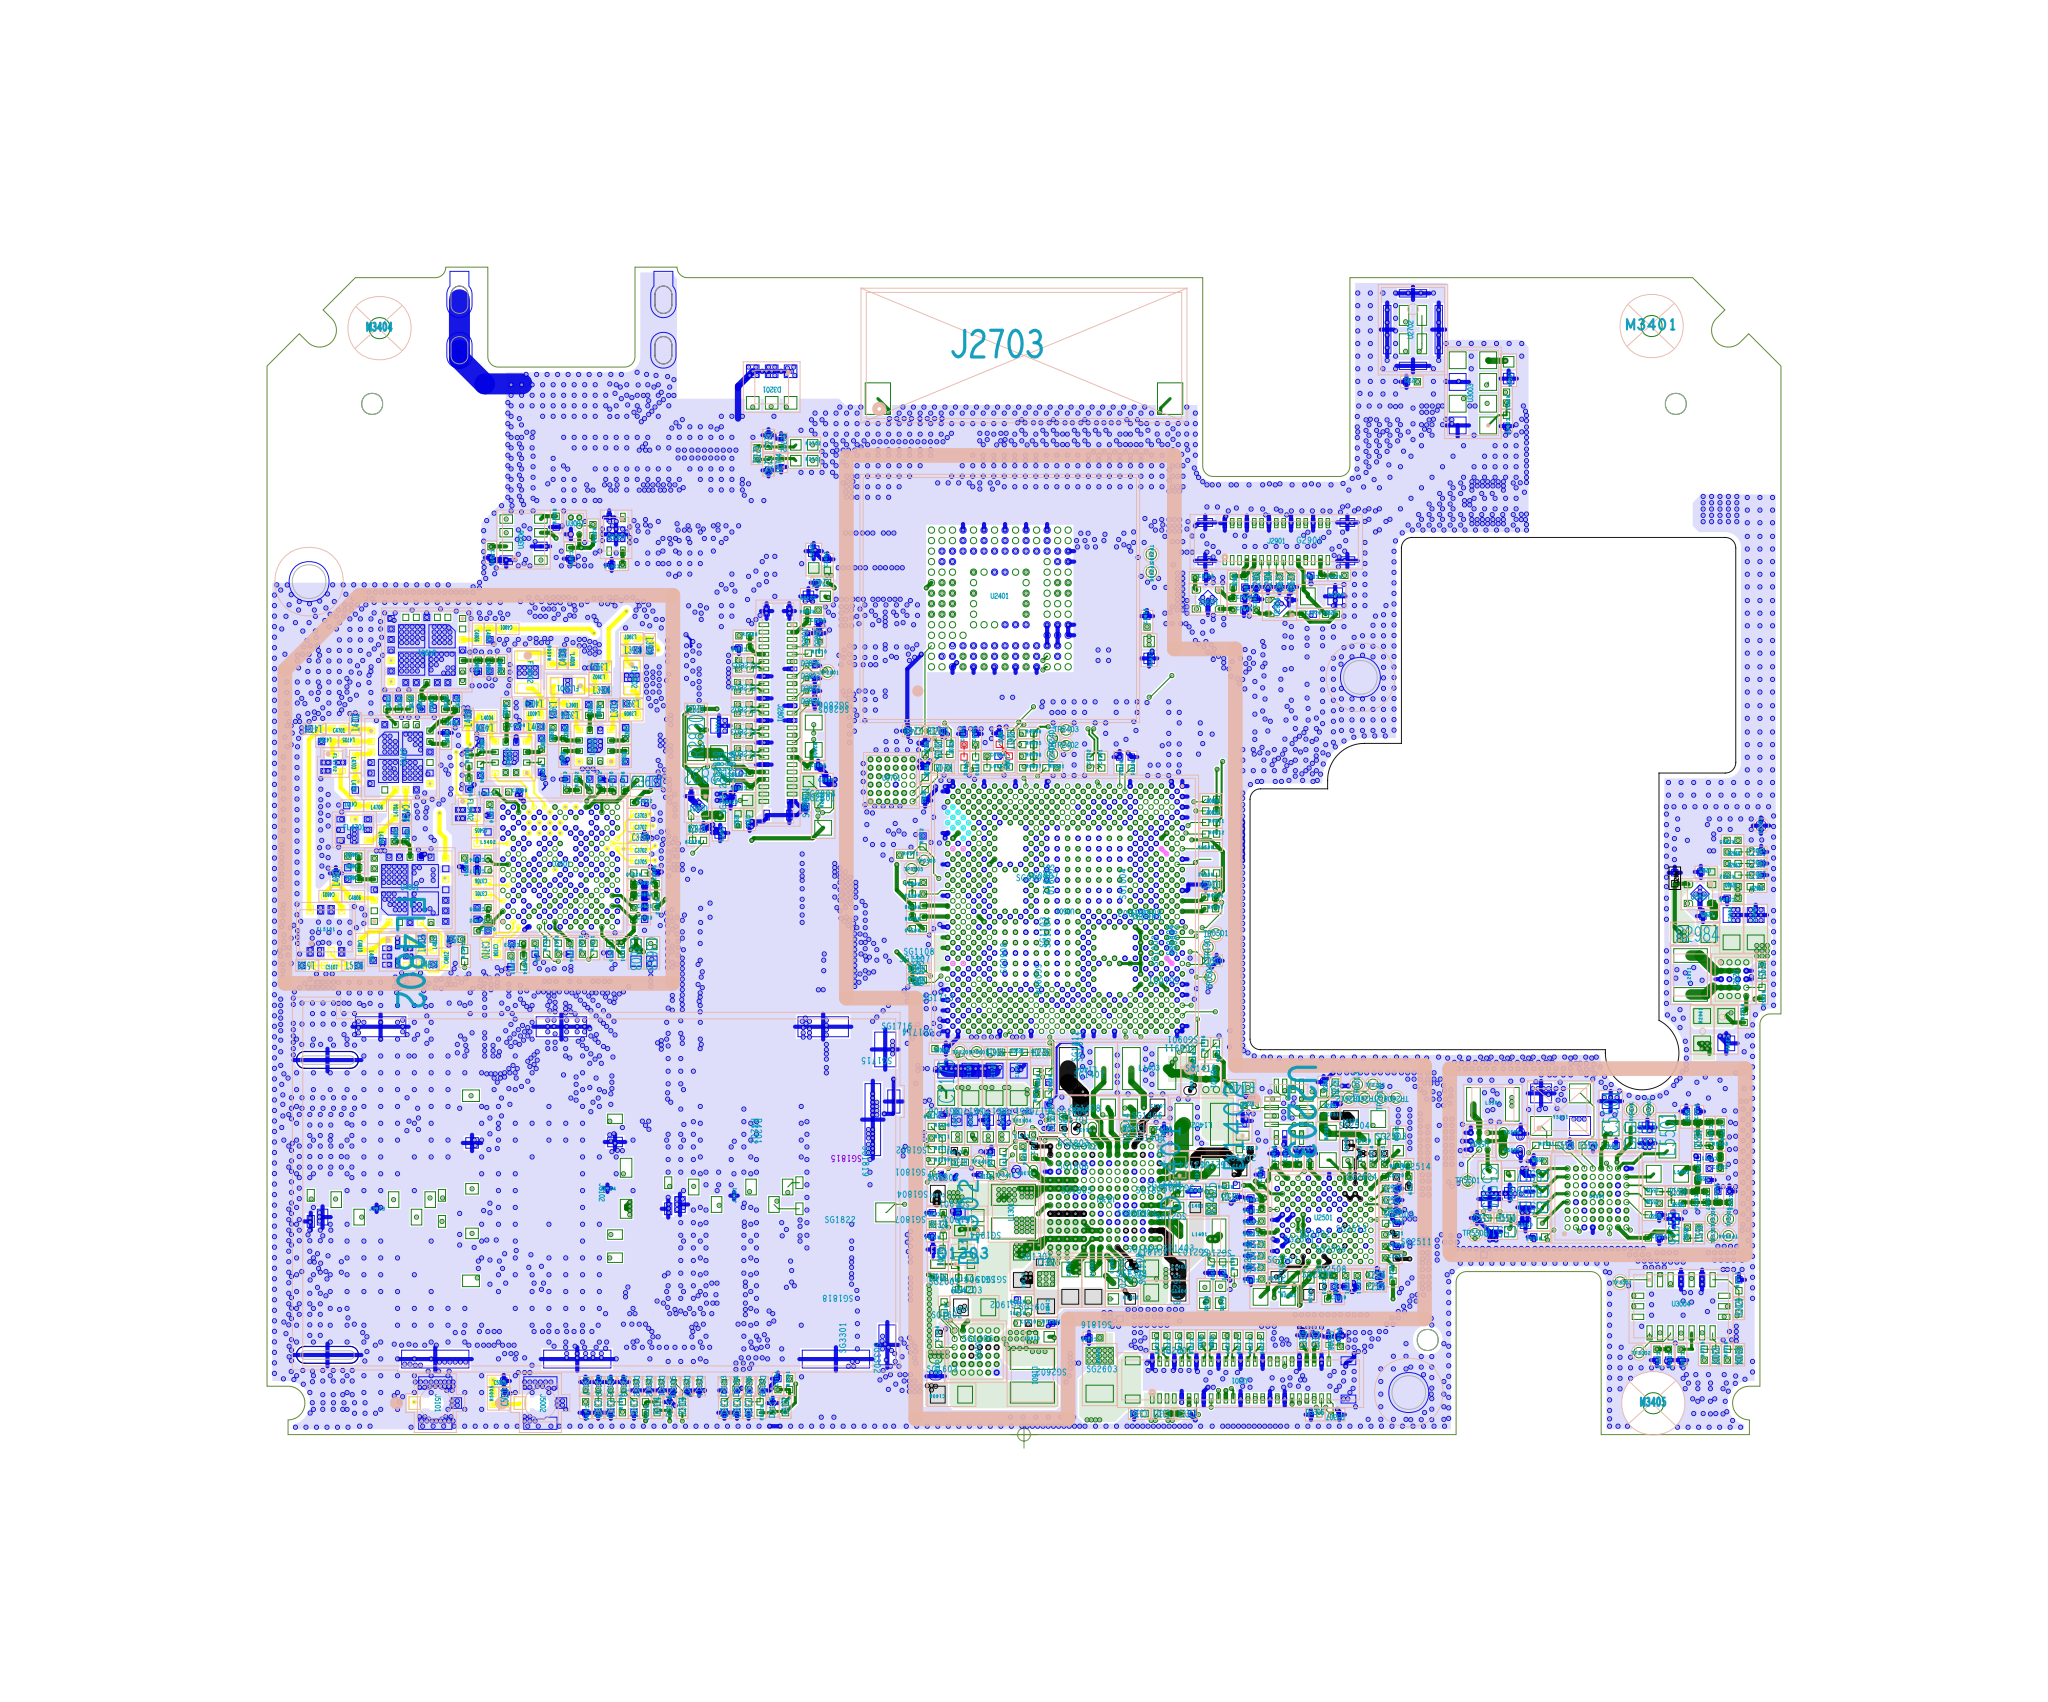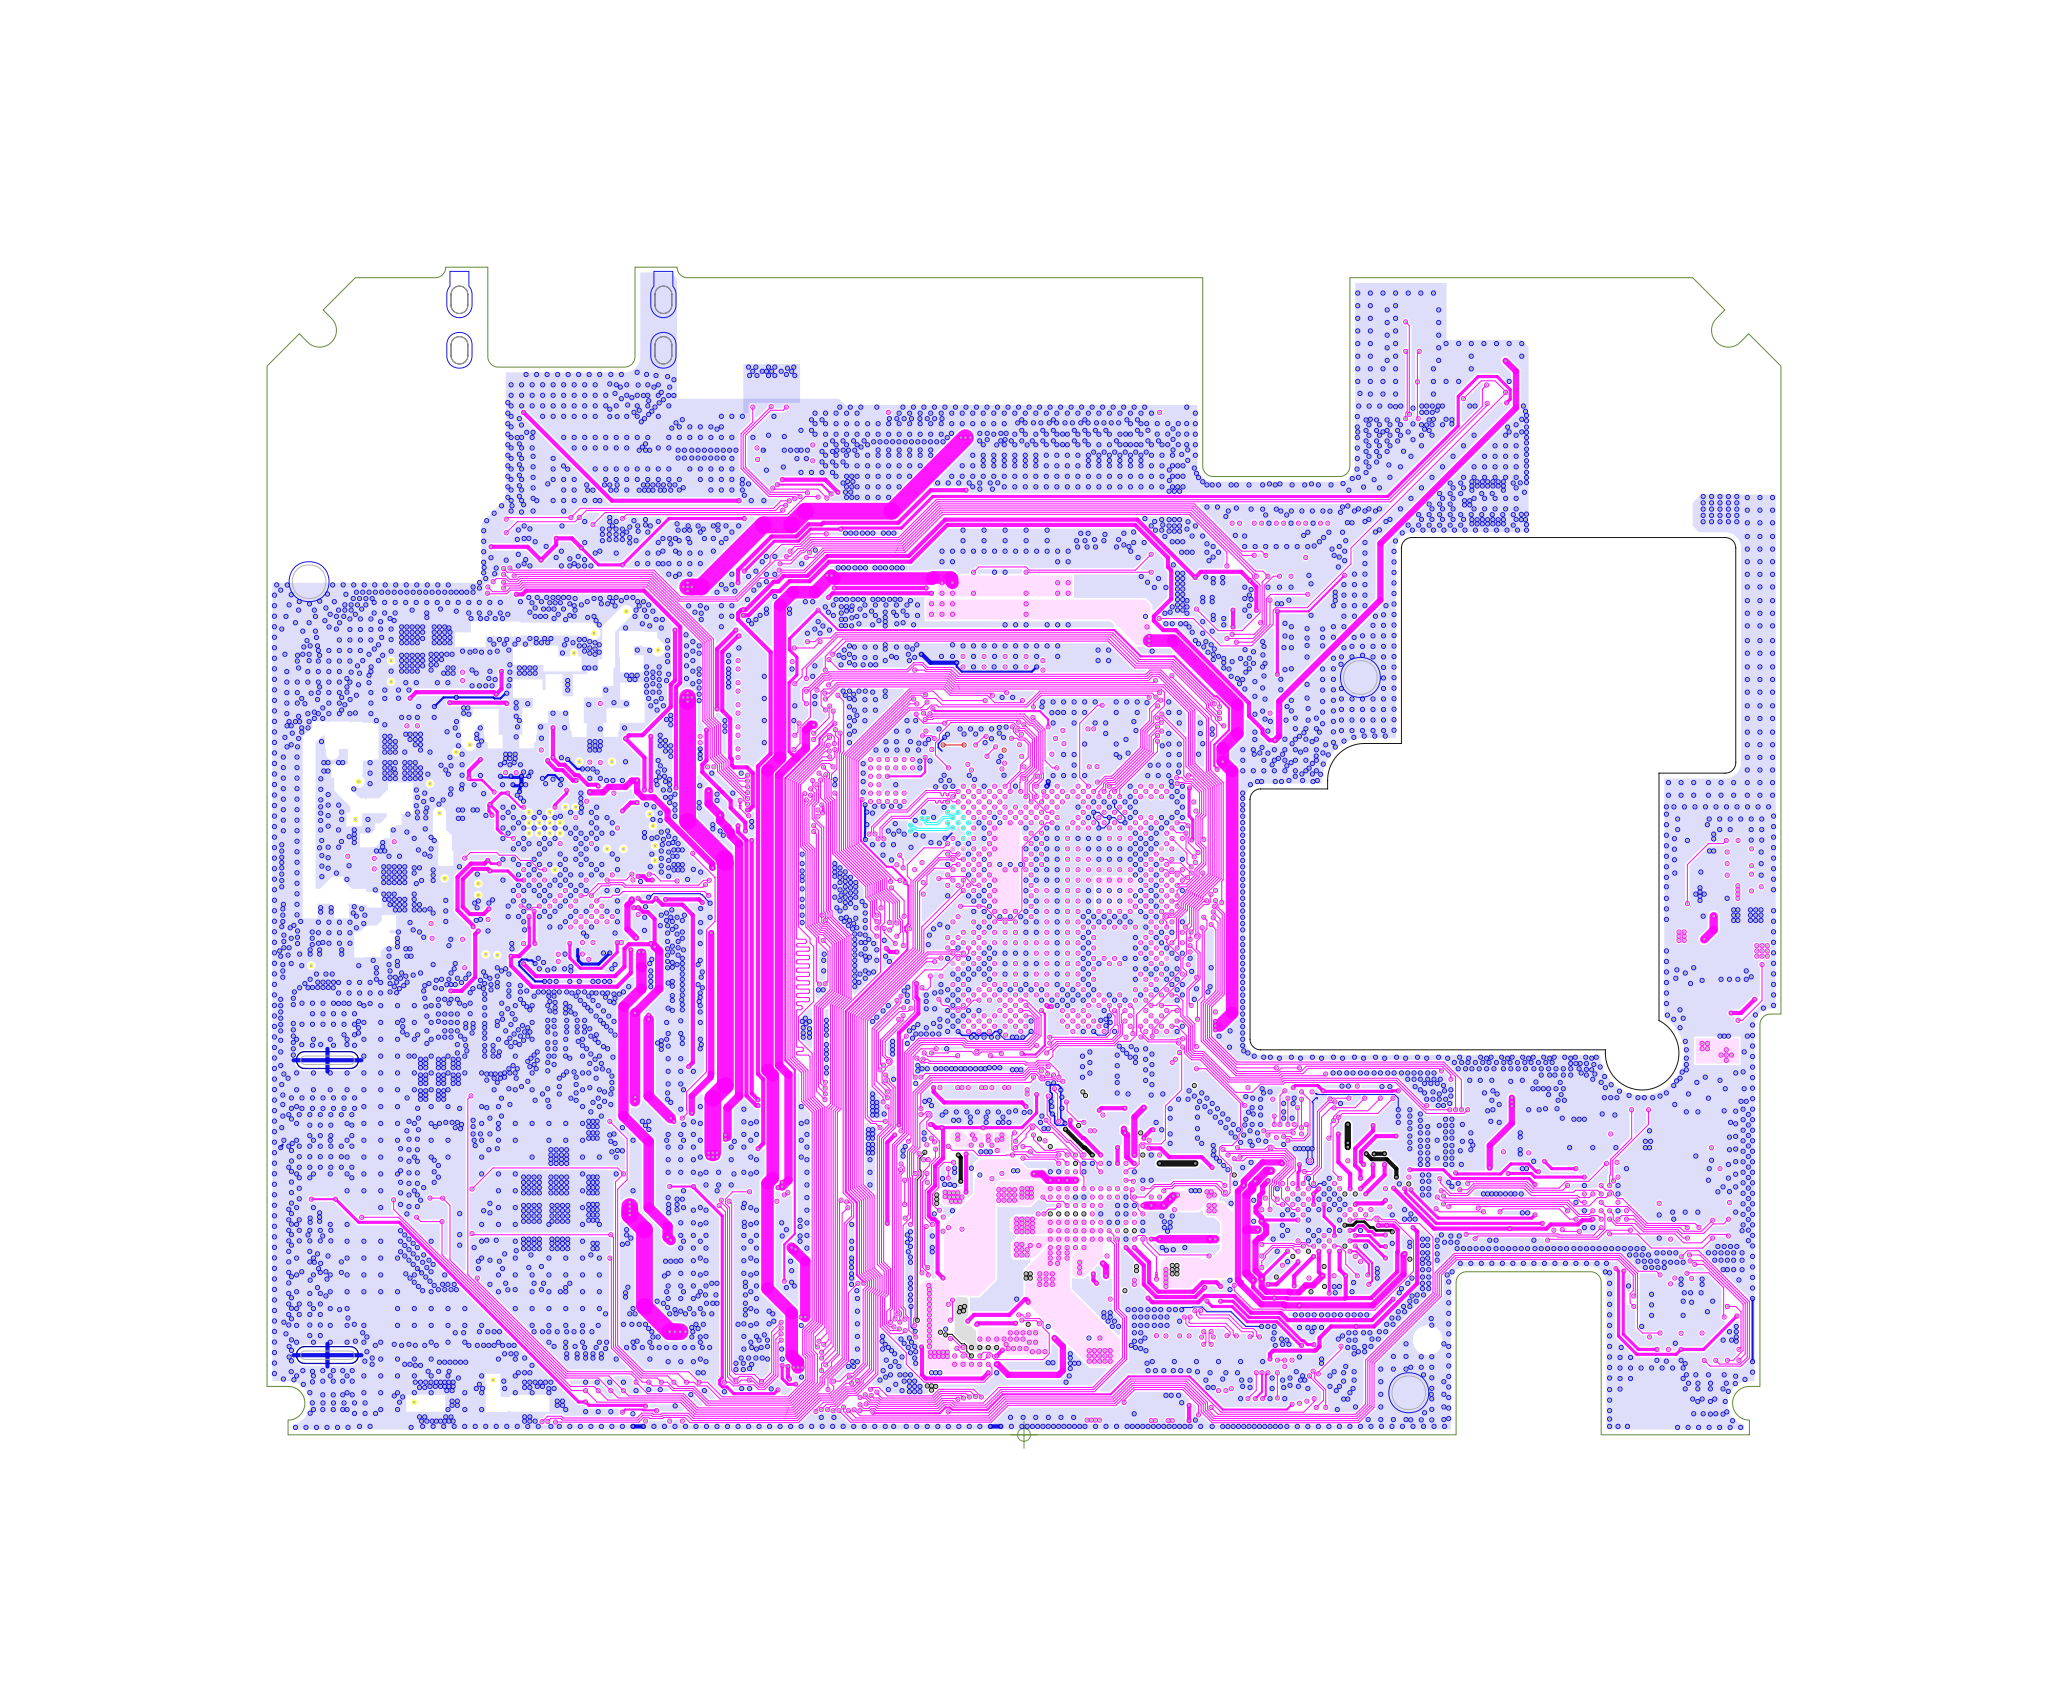Circuit board layout | Cadence Allegro
Layer stack:
# Cadence Allegro layer stack of  (unit mm; from the constraint file cross-section; dielectric type: 0 not recorded (Allegro does not mark core vs prepreg), 3 surface material)
index,name,kind,layer,copper_thickness_mm,dielectric_type,dielectric_thickness_mm,dielectric_material,dielectric_constant
0,Top Surface,other,,,,,,
1,Dielectric1,dielectric,,,3,0.02,FR-4,3.3
2,TOP,copper,TOP,0.024,,,,
3,Dielectric2,dielectric,,,0,0.05,FR-4,3.8
4,INNER LAYER 2,copper,INNER LAYER 2,0.02,,,,
5,Dielectric3,dielectric,,,0,0.05,FR-4,3.8
6,INNER LAYER 3,copper,INNER LAYER 3,0.02,,,,
7,Dielectric4,dielectric,,,0,0.05,FR-4,3.8
8,INNER LAYER 4,copper,INNER LAYER 4,0.02,,,,
9,Dielectric5,dielectric,,,0,0.05,FR-4,3.8
10,INNER LAYER 5,copper,INNER LAYER 5,0.02,,,,
11,Dielectric6,dielectric,,,0,0.064,FR-4,4.2
12,INNER LAYER 6,copper,INNER LAYER 6,0.02,,,,
13,Dielectric7,dielectric,,,0,0.05,FR-4,3.8
14,INNER LAYER 7,copper,INNER LAYER 7,0.02,,,,
15,Dielectric8,dielectric,,,0,0.05,FR-4,3.8
16,INNER LAYER 8,copper,INNER LAYER 8,0.02,,,,
17,Dielectric9,dielectric,,,0,0.05,FR-4,3.8
18,INNER LAYER 9,copper,INNER LAYER 9,0.02,,,,
19,Dielectric10,dielectric,,,0,0.05,FR-4,3.8
20,BOTTOM,copper,BOTTOM,0.024,,,,
21,Dielectric11,dielectric,,,3,0.02,FR-4,3.3
22,Bottom Surface,other,,,,,,
# drill layer pairs: low layer,high layer
drill_pair,TOP,BOTTOM
drill_pair,INNER LAYER 5,INNER LAYER 8
drill_pair,INNER LAYER 2,BOTTOM
drill_pair,INNER LAYER 8,INNER LAYER 9
drill_pair,TOP,INNER LAYER 6
drill_pair,TOP,INNER LAYER 7
drill_pair,INNER LAYER 7,BOTTOM
drill_pair,INNER LAYER 4,INNER LAYER 7
drill_pair,INNER LAYER 3,INNER LAYER 7
drill_pair,INNER LAYER 2,INNER LAYER 5
drill_pair,INNER LAYER 2,INNER LAYER 6
drill_pair,TOP,INNER LAYER 5
drill_pair,INNER LAYER 2,INNER LAYER 7
drill_pair,INNER LAYER 4,INNER LAYER 6
drill_pair,INNER LAYER 5,INNER LAYER 6
drill_pair,INNER LAYER 4,INNER LAYER 8
drill_pair,INNER LAYER 9,BOTTOM
drill_pair,INNER LAYER 6,INNER LAYER 7
drill_pair,INNER LAYER 3,INNER LAYER 9
drill_pair,INNER LAYER 2,INNER LAYER 4
drill_pair,INNER LAYER 4,INNER LAYER 9
drill_pair,INNER LAYER 3,INNER LAYER 6
drill_pair,INNER LAYER 5,INNER LAYER 7
drill_pair,INNER LAYER 5,BOTTOM
drill_pair,TOP,INNER LAYER 2
drill_pair,INNER LAYER 2,INNER LAYER 3
drill_pair,INNER LAYER 8,BOTTOM
drill_pair,INNER LAYER 2,INNER LAYER 9
drill_pair,INNER LAYER 3,INNER LAYER 5
drill_pair,INNER LAYER 6,INNER LAYER 8
drill_pair,INNER LAYER 7,INNER LAYER 9
drill_pair,TOP,INNER LAYER 9
drill_pair,TOP,INNER LAYER 4
drill_pair,INNER LAYER 5,INNER LAYER 9
drill_pair,INNER LAYER 4,INNER LAYER 5
drill_pair,INNER LAYER 7,INNER LAYER 8
drill_pair,TOP,INNER LAYER 8
drill_pair,TOP,INNER LAYER 3
drill_pair,INNER LAYER 6,INNER LAYER 9
drill_pair,INNER LAYER 6,BOTTOM
drill_pair,INNER LAYER 2,INNER LAYER 8
drill_pair,INNER LAYER 3,INNER LAYER 8
drill_pair,INNER LAYER 4,BOTTOM
drill_pair,INNER LAYER 3,BOTTOM
Part placement, first 452 of 1527 lines:
REFDES,COMP_VALUE,SYM_NAME,SYM_X,SYM_Y,SYM_ROTATE,SYM_MIRROR
B1501,600OHM/100MHZ,2P0402R,9.350,6.650,270.000,NO
B1502,600OHM/100MHZ,2P0402R,8.600,6.650,270.000,NO
B2501,120OHM/100MHZ,2P0402R,17.800,13.900,90.000,NO
B2502,1KOHM/100MHZ,2P0603R,14.450,13.700,90.000,NO
B2503,120OHM/100MHZ,2P0402R,16.550,14.050,180.000,NO
B2504,1KOHM/100MHZ,2P0603R,16.200,15.000,180.000,NO
B2505,1KOHM/100MHZ,2P0603R,11.900,6.550,0.000,NO
B2508,120OHM/100MHZ,2P0201R,18.000,12.850,180.000,NO
B4201,22OHM/100MHZ,2P0201R,-13.050,7.350,0.000,YES
C0503,DNI(10nF),2P0201R_DNI,8.900,22.525,0.000,NO
C0602,DNI(82PF),2P0201R_DNI,8.900,26.150,180.000,NO
C0603,22PF,2P0201R,-2.850,33.050,90.000,NO
C0604,22PF,2P0201R,-1.500,32.250,0.000,NO
C0605,22PF,2P0201R,-2.300,33.050,90.000,NO
C0606,22PF,2P0201R,-1.175,33.075,90.000,NO
C0701,0.1UF,2P0201R,3.700,31.950,90.000,NO
C0702,0.1UF,2P0201R,3.150,31.950,90.000,NO
C0703,0.1UF,2P0201R,-4.700,32.600,90.000,NO
C0902,1UF,2P0201R,4.400,29.400,180.000,YES
C0903,1UF,2P0201R,-1.850,20.450,270.000,YES
C0904,22UF,3PSM49X37N,4.000,22.510,90.000,YES
C0905,22UF,3PSM49X37N,5.400,24.110,90.000,YES
C0906,22UF,3PSM49X37N,5.400,22.510,90.000,YES
C0907,22UF,3PSM49X37N,4.000,24.110,90.000,YES
C0913,22UF,2P0603R,7.850,21.700,270.000,YES
C0914,1UF,2P0201R,6.950,21.050,90.000,YES
C0915,1UF,2P0201R,7.100,29.050,270.000,YES
C0916,1UF,2P0201R,-2.950,21.150,90.000,YES
C0917,1UF,2P0201R,-3.900,28.750,0.000,YES
C0918,220NF,2P0201R,-0.350,27.250,90.000,YES
C0922,22UF,3PSM49X37N,1.260,28.350,0.000,YES
C0923,22UF,3PSM49X37N,0.240,26.950,180.000,YES
C0924,22UF,3PSM49X37N,-3.750,24.940,270.000,YES
C0925,22UF,3PSM49X37N,7.100,26.740,270.000,YES
C0926,1UF,2P0201R,7.800,23.350,180.000,YES
C0927,1UF,2P0201R,7.300,26.150,0.000,YES
C0928,1UF,2P0201R,7.950,28.350,180.000,YES
C0929,1UF,2P0201R,7.800,23.900,180.000,YES
C0932,22UF,3PSM49X37N,-0.940,28.350,0.000,YES
C0933,22UF,3PSM49X37N,-0.940,26.950,0.000,YES
C0934,22UF,3PSM49X37N,-1.340,29.750,0.000,YES
C0935,22UF,3PSM49X37N,0.260,29.750,0.000,YES
C0936,22UF,3PSM49X37N,-0.760,25.550,180.000,YES
C0937,22UF,3PSM49X37N,-1.340,25.550,0.000,YES
C0938,22UF,3PSM49X37N,0.000,22.310,90.000,YES
C0939,22UF,3PSM49X37N,-1.400,22.310,90.000,YES
C0940,1UF,2P0201R,-0.600,23.150,270.000,YES
C0941,1UF,2P0201R,-0.050,23.150,270.000,YES
C0942,1UF,2P0201R,1.750,20.150,0.000,YES
C0944,1UF,2P0201R,-1.500,24.550,180.000,YES
C1002,1UF,2P0201R,3.050,29.350,270.000,YES
C1003,1UF,2P0201R,6.000,29.650,270.000,YES
C1004,1UF,2P0201R,0.950,20.450,90.000,YES
C1005,22UF,3PSM49X37N,4.890,25.900,180.000,YES
C1006,22UF,3PSM49X37N,-2.950,27.140,270.000,YES
C1010,1UF,2P0201R,5.300,29.650,270.000,YES
C1012,1UF,2P0201R,-0.350,28.500,90.000,YES
C1014,1UF,2P0201R,1.750,20.700,0.000,YES
C1015,22UF,3PSM49X37N,5.040,27.325,180.000,YES
C1016,22UF,3PSM49X37N,-2.340,23.550,0.000,YES
C1021,1UF,2P0201R,-1.750,23.700,90.000,YES
C1022,1UF,2P0201R,5.450,28.550,90.000,YES
C1023,1UF,2P0201R,4.900,28.550,90.000,YES
C1025,1UF,2P0201R,5.000,20.750,0.000,YES
C1026,1UF,2P0201R,-2.950,29.600,270.000,YES
C1029,1UF,2P0201R,6.400,21.050,90.000,YES
C1030,1UF,2P0201R,4.000,20.200,180.000,YES
C1031,1UF,2P0201R,2.200,28.900,0.000,YES
C1032,1UF,2P0201R,-2.950,22.300,90.000,YES
C1033,1UF,2P0201R,6.400,22.750,90.000,YES
C1041,1UF,2P0201R,6.700,21.850,180.000,YES
C1042,1UF,2P0201R,6.000,28.550,90.000,YES
C1043,1UF,2P0201R,-2.800,28.750,0.000,YES
C1044,1UF,2P0201R,-2.400,21.150,90.000,YES
C1045,220NF,2P0201R,6.475,25.900,270.000,YES
C1046,220NF,2P0201R,-2.400,22.300,90.000,YES
C1101,0.1UF,2P0201R,1.400,29.700,270.000,YES
C1102,1UF,2P0201R,0.850,29.700,270.000,YES
C1103,22UF,3PSM49X37N,1.090,23.700,180.000,YES
C1104,22UF,3PSM49X37N,1.861,27.929,180.000,YES
C1105,22UF,3PSM49X37N,1.840,26.500,180.000,YES
C1107,1UF,2P0201R,-2.575,24.550,0.000,YES
C1108,1UF,2P0201R,6.950,25.050,180.000,YES
C1109,1UF,2P0201R,5.850,20.350,90.000,YES
C1110,22UF,3PSM49X37N,1.090,25.100,180.000,YES
C1111,1UF,2P0201R,-0.700,20.450,90.000,YES
C1112,1UF,2P0201R,-0.150,20.450,90.000,YES
C1113,1UF,2P0201R,0.400,20.450,90.000,YES
C1114,1UF,2P0201R,2.500,29.700,270.000,YES
C1116,1UF,2P0201R,-1.500,22.900,180.000,YES
C1117,22UF,3PSM49X37N,0.990,21.700,180.000,YES
C1118,22UF,3PSM49X37N,3.850,25.860,90.000,YES
C1119,4.7UF,2P0402R,3.700,28.300,90.000,YES
C1120,1UF,2P0201R,4.350,28.550,90.000,YES
C1121,1UF,2P0201R,5.150,24.900,0.000,YES
C1124,1UF,2P0201R,-0.300,24.550,180.000,YES
C1125,1UF,2P0201R,3.650,27.000,270.000,YES
C1126,1UF,2P0201R,1.750,22.700,0.000,YES
C1127,22UF,2P0603R,5.950,18.650,90.000,YES
C1171,1UF,2P0201R,6.950,22.750,90.000,YES
C1172,1UF,2P0201R,6.550,28.600,270.000,YES
C1173,1UF,2P0201R,-1.200,23.700,90.000,YES
C1174,1UF,2P0201R,-0.300,24.000,180.000,YES
C1175,47UF,2P0603R,-3.700,16.650,90.000,NO
C1176,47UF,2P0603R,-8.350,16.850,0.000,YES
C1177,47UF,2P0603R,-6.650,20.500,270.000,YES
C1178,47UF,2P0603R,-8.350,15.700,0.000,YES
C1301,4.7UF,2P0603R,1.050,6.750,270.000,NO
C1302,DNI(33PF),2P0201R_DNI,1.000,8.200,0.000,NO
C1303,4.7UF,2P0603R,-0.100,8.000,270.000,NO
C1304,4.7UF,2P0603R,3.300,7.200,90.000,NO
C1305,0.027UF,2P0402R,4.250,7.600,90.000,NO
C1306,4.7UF,2P0603R,2.200,7.200,90.000,NO
C1307,22UF,2P0603R,-3.450,11.450,180.000,NO
C1308,4.7UF,2P0402R,-3.050,10.100,90.000,NO
C1309,10UF,2P0402RV1,0.475,12.500,180.000,NO
C1310,0.1UF,2P0201R,0.150,14.250,180.000,NO
C1311,1UF,2P0201R,0.500,13.450,90.000,NO
C1312,4.7UF,2P0402R,4.650,6.450,0.000,NO
C1313,220PF,2P0201R,-4.100,10.550,180.000,NO
C1314,220PF,2P0201R,1.900,7.500,0.000,YES
C1315,0.1UF,2P0201R,-2.850,7.450,180.000,NO
C1401,2.2UF,2P0402R,7.750,10.800,0.000,NO
C1402,4.7UF,2P0603R,9.600,12.700,0.000,NO
C1403,22UF,2P0603R,6.700,7.900,0.000,NO
C1404,22UF,2P0603R,6.700,6.750,0.000,NO
C1405,DNI(10UF),2P0402RV1_DNI,4.775,14.600,0.000,NO
C1406,2.2UF,2P0402R,7.750,11.550,0.000,NO
C1407,22UF,2P0603R,5.700,15.550,0.000,NO
C1408,10UF,2P0402RV1,7.900,17.175,270.000,NO
C1409,0.1UF,2P0201R,6.400,14.500,0.000,NO
C1410,22UF,2P0603R,3.350,15.550,180.000,NO
C1411,1500PF,2P0201R,1.850,14.850,270.000,NO
C1412,10UF,2P0402RV1,3.275,14.550,180.000,NO
C1413,82PF,2P0201R,10.500,13.550,0.000,NO
C1414,39PF,2P0201R,8.150,12.650,270.000,NO
C1419,1500PF,2P0201R,9.150,18.350,270.000,NO
C1501,22NF,2P0201R,9.450,7.950,270.000,NO
C1502,10UF,2P0402RV1,5.100,7.225,90.000,NO
C1503,0.1UF,2P0201R,5.800,11.800,180.000,YES
C1504,1UF,2P0201R,6.150,11.250,0.000,YES
C1505,0.1UF,2P0201R,6.750,9.100,90.000,YES
C1601,4.7UF,2P0603R,-2.350,6.050,180.000,NO
C1602,10UF,2P0402RV1,-4.200,3.625,270.000,NO
C1606,0.1UF,2P0201R,-4.050,4.550,90.000,NO
C1607,0.027UF,2P0402R,0.800,4.650,180.000,NO
C1608,22UF,2P0603R,-3.450,1.900,180.000,NO
C1610,1UF,2P0201R,-0.050,5.300,0.000,NO
C1701,47UF,2P0603R,-2.550,16.650,90.000,NO
C1702,47UF,2P0603R,-1.400,16.650,90.000,NO
C1703,2.2UF,2P0201R,2.150,13.800,270.000,YES
C1704,47UF,2P0603R,-0.250,16.650,90.000,NO
C1705,2.2UF,2P0201R,1.300,16.250,0.000,YES
C1706,2.2UF,2P0201R,0.200,16.250,0.000,YES
C1707,2.2UF,2P0201R,-0.900,16.250,0.000,YES
C1708,2.2UF,2P0201R,-2.000,16.250,0.000,YES
C1709,2.2UF,2P0201R,-3.100,16.250,0.000,YES
C1801,2.2UF,2P0201R,-5.000,13.600,90.000,YES
C1802,2.2UF,2P0201R,2.150,10.500,270.000,YES
C1803,22UF,2P0603R,4.150,6.900,90.000,YES
C1804,22UF,2P0603R,3.002,6.908,90.000,YES
C1805,2.2UF,2P0201R,-5.000,14.700,90.000,YES
C1806,2.2UF,2P0201R,2.150,11.600,270.000,YES
C1807,22UF,2P0603R,5.850,9.750,90.000,YES
C1808,2.2UF,2P0201R,2.150,12.700,270.000,YES
C1809,2.2UF,2P0201R,-5.000,11.400,90.000,YES
C1810,22UF,2P0603R,-7.550,8.250,90.000,YES
C1811,22UF,2P0603R,-8.700,8.250,90.000,YES
C1812,2.2UF,2P0201R,-5.000,12.500,90.000,YES
C1813,22UF,2P0603R,-8.700,11.100,90.000,YES
C1814,22UF,2P0603R,-8.700,13.500,270.000,YES
C1901,47UF,2P0603R,5.300,6.900,90.000,YES
C1903,0.1UF,2P0201R,-3.050,13.500,180.000,NO
C1904,1UF,2P0201R,-0.600,7.200,90.000,YES
C1905,4.7UF,2P0402R,-1.000,8.550,90.000,YES
C1906,1000PF,2P0201R,-3.450,6.950,0.000,YES
C1907,10UF,2P0402RV1,-1.800,9.025,90.000,YES
C1909,DNI(0.1uF),2P0201R_DNI,2.150,14.900,270.000,YES
C2001,4.7UF,2P0402R,-1.700,14.550,90.000,NO
C2002,1UF,2P0201R,-3.100,7.950,180.000,YES
C2003,1UF,2P0201R,-4.175,8.750,0.000,YES
C2004,4.7UF,2P0402R,-0.250,8.550,90.000,YES
C2005,4.7UF,2P0402R,-5.100,8.600,90.000,YES
C2006,4.7UF,2P0402R,-6.600,8.600,90.000,YES
C2007,4.7UF,2P0402R,-5.850,8.600,90.000,YES
C2008,4.7UF,2P0402R,5.700,16.550,270.000,YES
C2009,4.7UF,2P0402R,0.500,8.550,90.000,YES
C2010,4.7UF,2P0402R,-0.950,14.550,90.000,NO
C2011,2.2UF,2P0402R,-3.200,14.550,90.000,NO
C2012,2.2UF,2P0402R,-4.350,7.000,90.000,YES
C2013,2.2UF,2P0402R,1.650,8.200,0.000,YES
C2014,2.2UF,2P0402R,1.650,8.950,180.000,YES
C2015,2.2UF,2P0402R,-2.450,14.550,90.000,NO
C2016,1UF,2P0201R,-5.700,7.550,0.000,YES
C2017,1UF,2P0201R,-4.175,8.200,0.000,YES
C2018,1UF,2P0201R,-5.000,9.950,270.000,YES
C2019,DNI(1UF),2P0201R_DNI,-3.100,8.500,180.000,YES
C2020,1UF,2P0201R,-4.200,16.250,0.000,YES
C2021,1UF,2P0201R,-3.100,9.050,180.000,YES
C2022,4.7UF,2P0402R,-5.500,6.900,0.000,YES
C2101,47UF,2P0603R,11.650,9.650,180.000,YES
C2102,2.2UF,2P0201R,9.800,13.750,0.000,YES
C2103,47UF,2P0603R,11.650,13.450,180.000,YES
C2104,0.1UF,2P0201R,7.000,12.550,90.000,YES
C2105,2.2UF,2P0201R,9.850,9.350,0.000,YES
C2106,1UF,2P0201R,7.000,11.450,90.000,YES
C2107,2.2UF,2P0201R,8.750,9.350,0.000,YES
C2108,2.2UF,2P0201R,8.700,13.750,0.000,YES
C2201,0.1UF,2P0201R,-31.950,1.150,90.000,YES
C2202,0.1UF,2P0201R,-28.550,3.250,270.000,YES
C2204,0.1UF,2P0201R,14.250,16.500,90.000,NO
C2402,0.1UF,2P0201R,-9.350,41.350,90.000,NO
C2403,2.2UF,2P0402R,-10.000,41.600,90.000,NO
C2405,0.1UF,2P0201R,5.850,38.650,90.000,NO
C2406,2.2UF,2P0402R,5.950,37.300,270.000,NO
C2407,DNI(0.1uF),2P0201R_DNI,-9.600,40.500,180.000,NO
C2408,DNI(0.1uF),2P0201R_DNI,-5.250,33.450,180.000,NO
C2409,2.2UF,2P0402R,-9.850,39.850,180.000,NO
C2501,0.1UF,2P0201R,15.300,7.300,270.000,NO
C2502,DNI(330PF),2P0201R_DNI,17.450,11.150,0.000,NO
C2503,DNI(680pF),2P0201R_DNI,17.450,11.700,0.000,NO
C2504,DNI(680pF),2P0201R_DNI,17.450,10.600,0.000,NO
C2505,DNI(100PF),2P0201R_DNI,16.700,7.050,0.000,NO
C2506,DNI(100PF),2P0201R_DNI,16.700,7.600,0.000,NO
C2507,0.1UF,2P0201R,17.450,10.050,0.000,NO
C2509,4.7UF,2P0402R,15.400,13.350,90.000,NO
C2510,DNI(0.1uF),2P0201R_DNI,11.050,9.050,180.000,NO
C2511,0.47UF,2P0201R,15.850,7.300,270.000,NO
C2512,DNI(0.1uF),2P0201R_DNI,11.050,7.950,180.000,NO
C2513,1UF,2P0201R,14.500,15.150,0.000,NO
C2514,0.47UF,2P0201R,16.600,13.100,90.000,NO
C2515,0.47UF,2P0201R,17.150,13.100,90.000,NO
C2516,1UF,2P0201R,16.050,13.100,90.000,NO
C2518,0.1UF,2P0201R,14.750,7.300,270.000,NO
C2519,0.1UF,2P0201R,14.700,6.450,0.000,NO
C2520,0.47UF,2P0201R,17.450,12.250,0.000,NO
C2521,1UF,2P0201R,17.425,9.500,0.000,NO
C2522,4.7UF,2P0402R,12.400,7.500,180.000,NO
C2523,1UF,2P0201R,14.200,7.300,270.000,NO
C2524,4.7UF,2P0402R,13.550,7.050,270.000,NO
C2525,DNI(0.1uF),2P0201R_DNI,11.050,8.500,180.000,NO
C2527,0.1UF,2P0201R,17.450,8.400,0.000,NO
C2529,0.47UF,2P0201R,18.300,12.025,270.000,NO
C2601,0.1UF,2P0201R,11.050,11.250,180.000,NO
C2602,2.2UF,2P0201R,6.600,1.750,90.000,YES
C2603,0.1UF,2P0201R,11.050,10.150,180.000,NO
C2604,0.1UF,2P0201R,6.050,1.750,90.000,YES
C2605,10UF,2P0603R,2.950,4.600,90.000,YES
C2606,0.1UF,2P0201R,11.050,9.600,180.000,NO
C2607,22UF,2P0805R,1.550,2.650,270.000,YES
C2608,4.7UF,2P0603R,2.950,2.300,90.000,YES
C2609,1UF,2P0201R,7.050,2.800,180.000,YES
C2610,DNI(100PF),2P0201R_DNI,4.950,1.750,90.000,YES
C2611,DNI(100PF),2P0201R_DNI,3.850,1.750,90.000,YES
C2612,0.1UF,2P0201R,4.600,5.150,0.000,YES
C2613,22UF,2P0805R,-0.100,2.650,270.000,YES
C2614,0.1UF,2P0201R,11.050,10.700,180.000,NO
C2615,0.1UF,2P0201R,12.500,13.100,90.000,NO
C2616,0.1UF,2P0201R,17.450,8.950,0.000,NO
C2617,0.1UF,2P0201R,11.050,7.400,180.000,NO
C2618,0.1UF,2P0201R,11.950,13.100,90.000,NO
C2619,0.1UF,2P0201R,11.300,12.100,90.000,NO
C2620,0.1UF,2P0201R,13.050,13.100,90.000,NO
C2621,0.1UF,2P0201R,13.600,13.100,90.000,NO
C2701,DNI(33PF),2P0201R_DNI,-12.150,47.250,90.000,NO
C2702,DNI(33PF),2P0201R_DNI,-12.700,46.650,270.000,NO
C2703,DNI(33PF),2P0201R_DNI,-12.150,46.100,270.000,NO
C2722,0.1UF,2P0201R,18.450,50.050,180.000,NO
C2802,1UF,2P0201R,-10.050,38.650,0.000,NO
C2803,1UF,2P0201R,-10.050,31.750,0.000,NO
C2804,4.7UF,2P0402R,-13.550,30.150,180.000,NO
C2806,68PF,2P0201R,-13.300,31.450,180.000,NO
C2808,1UF,2P0201R,-13.300,37.400,180.000,NO
C2810,4.7UF,2P0402R,-9.850,31.050,0.000,NO
C2811,1UF,2P0603R,-14.500,33.050,90.000,NO
C2812,1UF,2P0201R,-13.300,30.800,180.000,NO
C2813,1UF,2P0402R,-14.450,29.000,270.000,NO
C2814,68PF,2P0201R,-13.050,29.250,270.000,NO
C2815,68PF,2P0201R,-10.375,30.125,270.000,NO
C2902,0.1UF,2P0201R,13.900,40.850,180.000,NO
C2903,DNI(33PF),2P0201R_DNI,11.050,40.550,90.000,NO
C2904,DNI(33PF),2P0201R_DNI,11.600,40.550,90.000,NO
C2905,DNI(33PF),2P0201R_DNI,12.150,40.550,270.000,NO
C2907,1UF,2P0201R,10.500,40.550,270.000,NO
C2908,DNI(33PF),2P0201R_DNI,12.700,40.550,270.000,NO
C2909,4.7UF,2P0603R,14.150,39.850,0.000,NO
C2910,1UF,2P0201R,12.850,32.700,180.000,YES
C2922,1UF,2P0201R,11.050,39.450,90.000,NO
C2926,1UF,2P0201R,13.500,39.000,0.000,NO
C2927,1UF,2P0201R,13.900,34.000,90.000,YES
C2929,DNI(33PF),2P0201R_DNI,6.350,34.900,90.000,YES
C2934,1UF,2P0201R,11.750,40.200,180.000,YES
C2935,DNI(33PF),2P0201R_DNI,11.750,38.550,180.000,YES
C2936,DNI(33PF),2P0201R_DNI,11.750,38.000,180.000,YES
C2937,0.1UF,2P0201R,11.750,39.650,180.000,YES
C2938,1UF,2P0201R,12.850,38.000,180.000,YES
C2939,0.1UF,2P0201R,12.850,38.550,180.000,YES
C2940,DNI(33PF),2P0201R_DNI,11.750,33.250,180.000,YES
C2941,1UF,2P0201R,11.750,33.800,180.000,YES
C2945,2.2UF,2P0201R,12.850,36.900,0.000,YES
C2946,1UF,2P0201R,10.200,39.200,0.000,NO
C2948,2.2UF,2P0201R,10.200,39.750,0.000,NO
C2951,1UF,2P0201R,11.750,36.300,0.000,YES
C2952,1UF,2P0201R,14.100,35.100,270.000,YES
C2953,1UF,2P0201R,8.400,40.750,0.000,NO
C2956,1UF,2P0201R,11.750,41.300,0.000,YES
C2959,1UF,2P0201R,12.850,39.400,0.000,YES
C2960,1UF,2P0201R,31.300,22.450,270.000,YES
C2961,0.1UF,2P0201R,31.050,23.250,0.000,YES
C2962,DNI(33PF),2P0201R_DNI,31.300,24.650,270.000,YES
C2963,1UF,2P0201R,35.200,22.250,90.000,YES
C2964,DNI(33PF),2P0201R_DNI,35.200,23.350,270.000,YES
C2965,DNI(33PF),2P0201R_DNI,34.800,27.700,0.000,NO
C2966,DNI(33PF),2P0201R_DNI,34.800,27.150,0.000,NO
C2967,DNI(33PF),2P0201R_DNI,34.800,26.600,0.000,NO
C2968,1UF,2P0201R,33.700,25.500,180.000,NO
C2969,1UF,2P0201R,32.550,24.650,180.000,NO
C2971,1UF,2P0201R,32.450,26.750,180.000,NO
C2972,1UF,2P0402R,32.350,18.850,0.000,YES
C2974,1UF,2P0201R,26.250,14.550,270.000,YES
C2975,1UF,2P0201R,28.700,14.300,180.000,YES
C2976,DNI(33PF),2P0201R_DNI,21.850,14.550,270.000,YES
C2977,1UF,2P0201R,21.300,14.550,270.000,YES
C2978,0.1UF,2P0201R,22.950,14.550,270.000,YES
C2979,DNI(33PF),2P0201R_DNI,24.050,14.550,270.000,YES
C2980,DNI(33PF),2P0201R_DNI,24.600,14.550,270.000,YES
C2981,DNI(33PF),2P0201R_DNI,19.600,10.900,0.000,YES
C2982,DNI(33PF),2P0201R_DNI,19.600,12.000,0.000,YES
C2983,22UF,2P0603R,34.800,24.050,90.000,NO
C2984,22UF,2P0603R,33.650,24.050,90.000,NO
C2985,10UF,2P0603R,33.400,19.250,270.000,NO
C2986,1UF,2P0201R,30.950,26.450,90.000,NO
C3001,0.1UF,2P0201R,31.250,3.800,270.000,NO
C3003,0.1UF,2P0201R,22.950,48.200,270.000,NO
C3004,4.7UF,2P0402R,23.050,50.600,270.000,NO
C3008,0.1UF,2P0201R,-25.350,41.950,270.000,NO
C3009,0.1UF,2P0201R,-21.600,41.900,270.000,NO
C3012,0.1UF,2P0201R,-19.350,41.350,180.000,NO
C3015,0.1UF,2P0201R,30.100,3.800,270.000,NO
C3016,1UF,2P0201R,30.650,3.800,270.000,NO
C3101,1UF,2P0201R,-11.700,2.400,90.000,NO
C3102,DNI(33PF),2P0201R_DNI,-13.650,1.300,270.000,NO
C3103,DNI(33PF),2P0201R_DNI,-14.250,1.300,270.000,NO
C3104,DNI(33PF),2P0201R_DNI,-13.100,1.300,270.000,NO
C3105,1UF,2P0201R,-20.850,1.300,270.000,NO
C3106,33PF,2P0201R,-17.050,4.850,0.000,YES
C3107,DNI(33PF),2P0201R_DNI,-18.550,1.300,270.000,NO
C3108,1UF,2P0201R,-15.950,4.850,180.000,YES
C3109,DNI(33PF),2P0201R_DNI,-20.250,1.300,270.000,NO
C3110,DNI(33PF),2P0201R_DNI,-19.650,1.300,270.000,NO
C3301,0.33UF,2P0201R,10.700,4.450,270.000,NO
C3302,DNI(10UF),2P0402RV1_DNI,-12.000,4.375,270.000,YES
C3303,1UF,2P0201R,-12.650,4.900,270.000,YES
C3304,33PF,2P0201R,-13.200,4.900,270.000,YES
C3306,DNI(33PF),2P0201R_DNI,-8.050,0.750,180.000,YES
C3307,0.1UF,2P0201R,9.600,4.450,270.000,NO
C3308,0.1UF,2P0201R,10.150,4.450,270.000,NO
C3309,0.33UF,2P0201R,11.250,4.450,270.000,NO
C3310,0.1UF,2P0201R,15.050,4.450,90.000,NO
C3311,DNI(33PF),2P0201R_DNI,6.600,1.000,180.000,NO
C3312,0.33UF,2P0201R,6.800,4.450,270.000,NO
C3313,DNI(33PF),2P0201R_DNI,7.700,1.000,0.000,NO
C3314,DNI(33PF),2P0201R_DNI,5.500,1.000,180.000,NO
C3315,DNI(33PF),2P0201R_DNI,13.872,4.463,90.000,NO
C3316,DNI(33PF),2P0201R_DNI,13.272,4.463,90.000,NO
C3317,0.1UF,2P0201R,7.350,4.450,270.000,NO
C3318,0.1UF,2P0201R,7.900,4.450,270.000,NO
C3319,0.33UF,2P0201R,6.250,4.450,270.000,NO
C3320,100PF,2P0201R,3.350,4.600,180.000,NO
C3321,0.1UF,2P0201R,10.150,3.650,180.000,YES
C3322,0.1UF,2P0201R,10.150,3.100,180.000,YES
C3323,DNI(1UF),2P0201R_DNI,11.400,1.900,0.000,YES
C3401,10NF,2P0402R,-31.700,37.200,0.000,YES
C3402,10NF,2P0402R,-31.700,37.950,0.000,YES
C3502,DNI(100PF),2P0201R_DNI,-27.000,23.550,180.000,NO
C3503,0.1UF,2P0201R,-18.300,24.500,0.000,NO
C3504,0.1UF,2P0201R,-21.600,23.100,270.000,NO
C3505,0.1UF,2P0201R,-17.500,26.450,90.000,NO
C3601,4.7UF,2P0402R,-17.950,31.050,0.000,NO
C3602,0.1UF,2P0201R,-25.750,24.500,180.000,NO
C3603,0.1UF,2P0201R,-18.300,25.600,0.000,NO
C3604,0.1UF,2P0201R,-25.750,27.400,180.000,NO
C3605,0.1UF,2P0201R,-25.750,25.050,180.000,NO
C3606,0.1UF,2P0201R,-19.000,30.900,90.000,NO
C3607,0.1UF,2P0201R,-24.400,22.500,270.000,NO
C3608,4.7UF,2P0402R,-18.450,22.900,270.000,NO
C3609,0.1UF,2P0201R,-24.250,30.550,0.000,NO
C3610,0.1UF,2P0201R,-19.550,30.900,90.000,NO
C3611,0.1UF,2P0201R,-25.350,30.550,180.000,NO
C3612,0.1UF,2P0201R,-20.100,30.900,90.000,NO
C3613,0.1UF,2P0201R,-21.750,30.900,90.000,NO
C3614,0.1UF,2P0201R,-20.650,30.900,90.000,NO
C3615,0.1UF,2P0201R,-19.700,23.100,270.000,NO
C3616,0.1UF,2P0201R,-25.400,29.700,270.000,NO
C3617,0.1UF,2P0201R,-25.750,26.850,180.000,NO
C3618,4.7UF,2P0402R,-17.700,22.900,270.000,NO
C3619,0.1UF,2P0201R,-23.250,23.100,270.000,NO
C3620,0.1UF,2P0201R,-25.750,23.950,0.000,NO
C3621,0.1UF,2P0201R,-18.300,25.050,0.000,NO
C3622,0.1UF,2P0201R,-18.300,30.050,0.000,NO
C3623,0.1UF,2P0201R,-24.100,23.350,180.000,NO
C3624,0.1UF,2P0201R,-18.300,26.150,0.000,NO
C3701,22PF,2P0201R,-25.750,25.650,180.000,NO
C3702,22PF,2P0201R,-18.300,27.850,0.000,NO
C3703,100PF,2P0201R,-18.300,29.500,0.000,NO
C3704,22PF,2P0201R,-25.050,23.100,270.000,NO
C3705,100PF,2P0201R,-18.300,27.300,0.000,NO
C3706,100PF,2P0201R,-25.750,26.250,180.000,NO
C3707,15PF,2P0201R,-18.300,28.950,0.000,NO
C3708,DNI(15PF),2P0201R_DNI,-18.300,28.400,0.000,NO
C3710,DNI(22PF),2P0201R_DNI,-25.600,23.100,270.000,NO
C3901,0.1UF,2P0201R,-20.700,34.450,90.000,NO
C3902,0.1UF,2P0201R,-21.850,33.350,90.000,NO
C3903,0.1UF,2P0201R,-18.950,33.350,90.000,NO
C4001,DNI(0.5PF),2P0201R_DNI,-29.550,31.750,0.000,YES
C4002,DNI(100PF),2P0201R_DNI,-26.700,32.950,90.000,YES
C4003,DNI(100PF),2P0201R_DNI,-24.450,33.300,180.000,YES
C4004,0.1UF,2P0201R,-24.350,33.650,0.000,NO
C4005,0.1UF,2P0201R,-26.400,30.950,270.000,NO
C4006,0.1UF,2P0201R,-25.850,32.700,90.000,NO
C4007,0.1UF,2P0201R,-22.950,32.850,90.000,NO
C4008,DNI(0.5PF),2P0201R_DNI,-21.950,36.900,90.000,NO
C4010,DNI(22PF),2P0201R_DNI,-20.850,33.600,270.000,YES
C4011,0.1UF,2P0201R,-20.100,30.200,90.000,YES
C4012,22PF,2P0201R,-23.350,33.350,0.000,YES
C4013,22PF,2P0201R,-19.800,31.600,180.000,YES
C4014,0.1UF,2P0201R,-19.800,31.050,180.000,YES
C4015,DNI(1.2PF),2P0201R_DNI,-19.200,32.500,270.000,YES
C4202,22UF,2P0603R,-14.750,7.100,180.000,YES
C4203,1UF,2P0201R,-12.700,11.750,90.000,YES
C4204,10UF,2P0402RV1,-13.625,12.350,0.000,YES
C4205,470PF,2P0201R,-16.500,10.950,180.000,YES
C4206,1UF,2P0201R,-12.700,10.675,90.000,YES
C4207,1UF,2P0201R,-12.700,9.600,270.000,YES
C4208,1UF,2P0201R,-16.200,13.650,270.000,YES
C4210,22PF,2P0201R,-11.900,13.750,90.000,YES
C4211,DNI(100PF),2P0201R_DNI,-18.650,10.700,0.000,YES
C4212,DNI(100PF),2P0201R_DNI,-18.650,10.150,0.000,YES
C4213,4.7UF,2P0402R,-16.350,12.100,270.000,YES
C4220,22UF,2P0603R,-16.500,8.300,90.000,YES
C4301,0.1UF,2P0201R,-13.900,18.450,90.000,YES
C4302,2.2UF,2P0201R,-13.350,18.450,90.000,YES
C4303,0.1UF,2P0201R,-18.600,19.150,0.000,YES
C4304,2.2UF,2P0201R,-18.600,18.600,0.000,YES
C4305,1.2PF,2P0201R,-17.550,20.550,0.000,YES
C4306,1.5PF,2P0201R,-16.450,21.100,0.000,YES
C4307,1.2PF,2P0201R,-13.850,16.550,180.000,YES
C4308,1.2PF,2P0201R,-16.050,16.600,0.000,YES
C4309,0.1UF,2P0201R,-13.650,19.350,180.000,YES
C4310,DNI(0.1uF),2P0201R_DNI,-16.900,16.350,90.000,YES
C4401,0.1UF,2P0201R,-18.650,14.050,180.000,YES
Pad and via stacks, first 94 of 565 lines:
# Allegro (Cadence) via spans and padstacks; design units: ("millimeters" 3 1000)
# via spans: padstack,start_layer,end_layer,net_example,count
5-8,ETCH/INNER LAYER 5,ETCH/INNER LAYER 8,GND,22
2-BOTTOM,ETCH/INNER LAYER 2,ETCH/BOTTOM,GND,363
8-9,ETCH/INNER LAYER 8,ETCH/INNER LAYER 9,VREG_LVS2A_1P8,432
TOP-6,ETCH/TOP,ETCH/INNER LAYER 6,N48287053,175
TOP-7,ETCH/TOP,ETCH/INNER LAYER 7,GND,655
7-BOTTOM,ETCH/INNER LAYER 7,ETCH/BOTTOM,GND,1575
4-7,ETCH/INNER LAYER 4,ETCH/INNER LAYER 7,GND,23
3-7,ETCH/INNER LAYER 3,ETCH/INNER LAYER 7,GND,1587
2-5,ETCH/INNER LAYER 2,ETCH/INNER LAYER 5,GND,96
2-6,ETCH/INNER LAYER 2,ETCH/INNER LAYER 6,VREG_L3A_1P0,143
TOP-5,ETCH/TOP,ETCH/INNER LAYER 5,GND,1535
2-7,ETCH/INNER LAYER 2,ETCH/INNER LAYER 7,VREG_L11A_1P0,9
4-6,ETCH/INNER LAYER 4,ETCH/INNER LAYER 6,RF_CLK1,246
5-6,ETCH/INNER LAYER 5,ETCH/INNER LAYER 6,GND,77
4-8,ETCH/INNER LAYER 4,ETCH/INNER LAYER 8,VPA_0,79
9-BOTTOM,ETCH/INNER LAYER 9,ETCH/BOTTOM,VREG_LVS2A_1P8,1623
6-7,ETCH/INNER LAYER 6,ETCH/INNER LAYER 7,VREG_S7A_1P025,33
3-9,ETCH/INNER LAYER 3,ETCH/INNER LAYER 9,GND,12
2-4,ETCH/INNER LAYER 2,ETCH/INNER LAYER 4,VREG_L8A_1P2,313
4-9,ETCH/INNER LAYER 4,ETCH/INNER LAYER 9,ACCEL_INT,23
3-6,ETCH/INNER LAYER 3,ETCH/INNER LAYER 6,GND,16
5-7,ETCH/INNER LAYER 5,ETCH/INNER LAYER 7,GND,444
VIA-INNER_LAYER_5-BOTTOM,ETCH/INNER LAYER 5,ETCH/BOTTOM,GND,2548
TOP-2,ETCH/TOP,ETCH/INNER LAYER 2,N35372594,717
2-3,ETCH/INNER LAYER 2,ETCH/INNER LAYER 3,GND,5
8-BOTTOM,ETCH/INNER LAYER 8,ETCH/BOTTOM,MSM_JTAG_SRST_N,668
2-9,ETCH/INNER LAYER 2,ETCH/INNER LAYER 9,SSC_SPI1_MISO,23
3-5,ETCH/INNER LAYER 3,ETCH/INNER LAYER 5,GND,813
6-8,ETCH/INNER LAYER 6,ETCH/INNER LAYER 8,MSM_JTAG_SRST_N,110
7-9,ETCH/INNER LAYER 7,ETCH/INNER LAYER 9,VPH_PWR,54
TOP-BOTTOM,ETCH/TOP,ETCH/BOTTOM,GND,1806
TOP-9,ETCH/TOP,ETCH/INNER LAYER 9,GND,162
TOP-4,ETCH/TOP,ETCH/INNER LAYER 4,VREG_S4A_1P8_DIG,454
5-9,ETCH/INNER LAYER 5,ETCH/INNER LAYER 9,GND,7
4-5,ETCH/INNER LAYER 4,ETCH/INNER LAYER 5,GND,39
7-8,ETCH/INNER LAYER 7,ETCH/INNER LAYER 8,GND,96
TOP-8,ETCH/TOP,ETCH/INNER LAYER 8,GND,426
TOP-3,ETCH/TOP,ETCH/INNER LAYER 3,GND,2254
6-9,ETCH/INNER LAYER 6,ETCH/INNER LAYER 9,VREG_S4A_1P8_DIG,69
6-BOTTOM,ETCH/INNER LAYER 6,ETCH/BOTTOM,MSM_JTAG_TMS,208
2-8,ETCH/INNER LAYER 2,ETCH/INNER LAYER 8,GND,53
3-8,ETCH/INNER LAYER 3,ETCH/INNER LAYER 8,GND,66
4-BOTTOM,ETCH/INNER LAYER 4,ETCH/BOTTOM,RFFE4_DATA,80
3-BOTTOM,ETCH/INNER LAYER 3,ETCH/BOTTOM,GND,131
# Allegro padstack definitions: name,start_layer,end_layer,drill,plating,holeType,type
SMD50X50,"ETCH/TOP","ETCH/TOP",0.0,"NON_PLATED","none","smd"
MS7X8PRD,"ETCH/TOP","ETCH/TOP",0.0,"NON_PLATED","none","smd"
SMDS0_3X0_3,"ETCH/TOP","ETCH/TOP",0.0,"NON_PLATED","none","smd"
MS54X99PRD,"ETCH/TOP","ETCH/TOP",0.0,"NON_PLATED","none","smd"
MS97X99PRD,"ETCH/TOP","ETCH/TOP",0.0,"NON_PLATED","none","smd"
MS6X6PRD,"ETCH/TOP","ETCH/TOP",0.0,"NON_PLATED","none","smd"
MS25X2PRDODD,"ETCH/TOP","ETCH/TOP",0.0,"NON_PLATED","none","smd"
MS25X2PRDODDV1,"ETCH/TOP","ETCH/TOP",0.0,"NON_PLATED","none","smd"
MS2X25CHBRPRDODD,"ETCH/TOP","ETCH/TOP",0.0,"NON_PLATED","none","smd"
MS2X25CHBLPRDODD,"ETCH/TOP","ETCH/TOP",0.0,"NON_PLATED","none","smd"
MS2X25CHTLPRDODD,"ETCH/TOP","ETCH/TOP",0.0,"NON_PLATED","none","smd"
MS2X25CHTRPRDODD,"ETCH/TOP","ETCH/TOP",0.0,"NON_PLATED","none","smd"
MS3X8PRD,"ETCH/TOP","ETCH/TOP",0.0,"NON_PLATED","none","smd"
MS4X8PRD,"ETCH/TOP","ETCH/TOP",0.0,"NON_PLATED","none","smd"
MS1_2X2_0NSP,"ETCH/TOP","ETCH/TOP",0.0,"NON_PLATED","none","smd"
MS2X65PRD,"ETCH/TOP","ETCH/TOP",0.0,"NON_PLATED","none","smd"
MS2X5PRD,"ETCH/TOP","ETCH/TOP",0.0,"PLATED","none","smd"
MS9X92CHTLPRD,"ETCH/TOP","ETCH/TOP",0.0,"NON_PLATED","none","smd"
MS9X92CHTRPRD,"ETCH/TOP","ETCH/TOP",0.0,"NON_PLATED","none","smd"
MS9X92CHBRPRD,"ETCH/TOP","ETCH/TOP",0.0,"NON_PLATED","none","smd"
MS9X92CHBLPRD,"ETCH/TOP","ETCH/TOP",0.0,"NON_PLATED","none","smd"
MS5X2_5PRDNSP,"ETCH/TOP","ETCH/TOP",0.0,"NON_PLATED","none","smd"
MS9X92CHTL3PRD,"ETCH/TOP","ETCH/TOP",0.0,"PLATED","none","smd"
MS9X92CHTR3PRD,"ETCH/TOP","ETCH/TOP",0.0,"PLATED","none","smd"
MS9X92CHBR3PRD,"ETCH/TOP","ETCH/TOP",0.0,"PLATED","none","smd"
MS9X92CHBL3PRD,"ETCH/TOP","ETCH/TOP",0.0,"PLATED","none","smd"
MS65X1_6PRD,"ETCH/TOP","ETCH/TOP",0.0,"PLATED","none","smd"
MS1_0RDM3_0RDNSP,"ETCH/TOP","ETCH/TOP",0.0,"PLATED","none","smd"
MS8X1_3PRD,"ETCH/TOP","ETCH/TOP",0.0,"NON_PLATED","none","smd"
SMDS0_3-SHIELD,"ETCH/TOP","ETCH/TOP",0.0,"NON_PLATED","none","smd"
BALL20,"ETCH/TOP","ETCH/TOP",0.0,"NON_PLATED","none","smd"
CIRCLE1_3,"ETCH/TOP","ETCH/TOP",0.0,"NON_PLATED","none","smd"
MS25RDM3RDP26RD,"ETCH/TOP","ETCH/TOP",0.0,"PLATED","none","smd"
PAD5,"ETCH/TOP","ETCH/TOP",0.0,"NON_PLATED","none","smd"
MS25M3RDP27X27RD,"ETCH/TOP","ETCH/TOP",0.0,"PLATED","none","smd"
PAD52,"ETCH/TOP","ETCH/TOP",0.0,"NON_PLATED","none","smd"
MS3RDP32X32RD,"ETCH/TOP","ETCH/TOP",0.0,"NON_PLATED","none","smd"
MS22RDM28RDP198X198RD,"ETCH/TOP","ETCH/TOP",0.0,"NON_PLATED","none","smd"
MS89X1_05ODD,"ETCH/TOP","ETCH/TOP",0.0,"NON_PLATED","none","smd"
MS4X3CHBRPRD,"ETCH/TOP","ETCH/TOP",0.0,"NON_PLATED","none","smd"
MS4X3CHBLPRD,"ETCH/TOP","ETCH/TOP",0.0,"NON_PLATED","none","smd"
MS4X3CHTRPRD,"ETCH/TOP","ETCH/TOP",0.0,"NON_PLATED","none","smd"
MS4X3CHTLPRD,"ETCH/TOP","ETCH/TOP",0.0,"NON_PLATED","none","smd"
MS4X4P35X35RD,"ETCH/TOP","ETCH/TOP",0.0,"PLATED","none","smd"
MS3X4P27X4RD,"ETCH/TOP","ETCH/TOP",0.0,"NON_PLATED","none","smd"
MS4X3P4X27RD,"ETCH/TOP","ETCH/TOP",0.0,"PLATED","none","smd"
MS72X75PRD,"ETCH/TOP","ETCH/TOP",0.0,"NON_PLATED","none","smd"
Design rules, without the lines most boards share, first 7 of 248 lines:
# Cadence Allegro design rules of  (from the Constraint Manager export constraints.dcfx, design unit mm; typed fields in mm)
# columns: name | kind | enabled | priority | scope1 | scope2 | descriptor | typed fields (field=value)
# Allegro precedence (priority 1 wins): 1 Region class-to-class, 2 Region class, 3 Region, 4 class-to-class, 5 DiffPair/Bus/NetGroup override, 6 NetClass, 7 constraint set (CSet) default
# per-layer values are written LAYER=value in the descriptor and LAYER:mm in the typed field; a maximum of 0 means no limit set
# --- net classes (and buses / net groups) ---
GND-ALL | NetClass | enabled | 6 | GND | All | Net Class (PhysicalCSet=PWR) (members: 1 Net) | physicalcset=PWR
RF_50OHM | NetClass | enabled | 6 | GNSS_IN, N48158912, N49012543, N49033316, N49041493, N49212510, N49305713, N49307488, PRX_ANT, WL_5G_CH1_B46_DRX, WTR_DRX_LAA, WTR_DRX_LB, WTR_DRX_MB_A, WTR_DRX_MB_B, WTR_DRX_UHB, WTR_PRX_LAA, WTR_PRX_LB, WTR_PRX_MB_A, WTR_PRX_MB_B, WTR_PRX_UHB, WTR0_TX_CH1_LMB1, WTR0_TX_CH1_LMB2, 600MHZ_LNA_IN, WTR_DRX_HB, WTR_DRX_LHB, WTR_PRX_HB, WTR_PRX_LHB, WTR_RX_TXFB_P, N50673167, CPL_HB, CPL_MB, CPL_UHB, N50017840, N50017842, N50047887, B1/B3/B7/B41_MIMO_CH1, B7/B41_MIMO_CH0, N49012494, B42_DRX_CH1, DRX_ANT, DRX_FLT_B27, DRX_FLT_B71, DRX_LNA_B27, DRX_LNA_B71, MB_B7_MIMO, MB_B41_MIMO, MB_LNA_AUX2_B7_RX, MB_LNA_AUX2_B41_RX, M592_MB_DRX_ANT, M610_LB_DRX_ANT, N35858069, N47951961, N47951964, N47951977, N47952018, N47952028, N48051262, N48051304, N48051430, N48051470, N48121397, N48121407, N48121496, N48121509, N48122336, N48220803, N48221715, N48221875, N48221877, N48222160, N48222212, N48222214, N48223922, N48224363, N48227004, N48227022, N48227420, N48227432, N48230925, N48231137, N48251103, N48251195, N48251217, N48251297, N48251303, N48256362, N48256741, N48257169, N48257796, N48287053, N48287590 | All | Net Class (PhysicalCSet=RF_50OHM) (SpacingCSet=RF_50OHM) (members: 2 Xnet, 89 Net) | physicalcset=RF_50OHM spacingcset=RF_50OHM